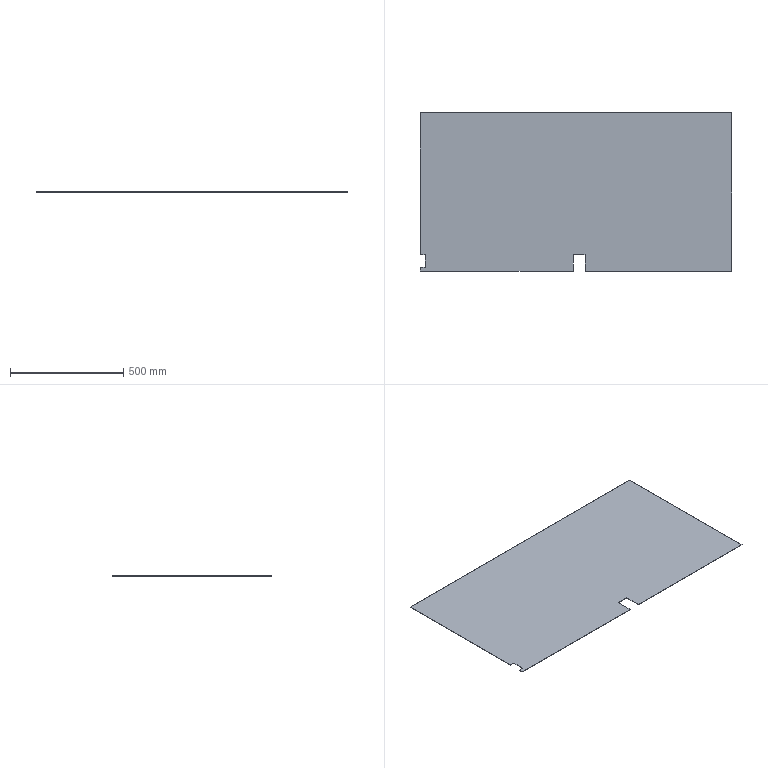Part | SolidWorks | 1 solid | 14 faces | box 1374 x 700 x 1.5 mm | volume 1435242 mm3 | plane 14
STEP:
#1=CARTESIAN_POINT('',(-687.,350.,0.));
#2=VERTEX_POINT('',#1);
#3=CARTESIAN_POINT('',(-687.,-277.,0.));
#4=VERTEX_POINT('',#3);
#5=CARTESIAN_POINT('',(-687.,-350.,0.));
#6=DIRECTION('',(0.,-1.,0.));
#7=VECTOR('',#6,1000.);
#8=LINE('',#5,#7);
#9=EDGE_CURVE('',#2,#4,#8,.T.);
#10=ORIENTED_EDGE('',*,*,#9,.T.);
#11=CARTESIAN_POINT('',(-687.,-277.,1.5));
#12=VERTEX_POINT('',#11);
#13=CARTESIAN_POINT('',(-687.,-277.,-0.001));
#14=DIRECTION('',(0.,0.,-1.));
#15=VECTOR('',#14,1000.);
#16=LINE('',#13,#15);
#17=EDGE_CURVE('',#12,#4,#16,.T.);
#18=ORIENTED_EDGE('',*,*,#17,.F.);
#19=CARTESIAN_POINT('',(-687.,350.,1.5));
#20=VERTEX_POINT('',#19);
#21=CARTESIAN_POINT('',(-687.,-350.,1.5));
#22=DIRECTION('',(0.,-1.,0.));
#23=VECTOR('',#22,1000.);
#24=LINE('',#21,#23);
#25=EDGE_CURVE('',#20,#12,#24,.T.);
#26=ORIENTED_EDGE('',*,*,#25,.F.);
#27=CARTESIAN_POINT('',(-687.,350.,1.5));
#28=DIRECTION('',(0.,0.,-1.));
#29=VECTOR('',#28,1000.);
#30=LINE('',#27,#29);
#31=EDGE_CURVE('',#20,#2,#30,.T.);
#32=ORIENTED_EDGE('',*,*,#31,.T.);
#33=EDGE_LOOP('',(#10,#18,#26,#32));
#34=FACE_OUTER_BOUND('',#33,.T.);
#35=CARTESIAN_POINT('',(-687.,-350.,1.5));
#36=DIRECTION('',(1.,0.,0.));
#37=DIRECTION('',(0.,0.,-1.));
#38=AXIS2_PLACEMENT_3D('',#35,#36,#37);
#39=PLANE('',#38);
#40=ADVANCED_FACE('',(#34),#39,.F.);
#41=CARTESIAN_POINT('',(-687.,-350.,0.));
#42=VERTEX_POINT('',#41);
#43=CARTESIAN_POINT('',(-12.,-350.,0.));
#44=VERTEX_POINT('',#43);
#45=CARTESIAN_POINT('',(687.,-350.,0.));
#46=DIRECTION('',(1.,0.,0.));
#47=VECTOR('',#46,1000.);
#48=LINE('',#45,#47);
#49=EDGE_CURVE('',#42,#44,#48,.T.);
#50=ORIENTED_EDGE('',*,*,#49,.T.);
#51=CARTESIAN_POINT('',(-12.,-350.,1.5));
#52=VERTEX_POINT('',#51);
#53=CARTESIAN_POINT('',(-12.,-350.,-0.001));
#54=DIRECTION('',(0.,0.,-1.));
#55=VECTOR('',#54,1000.);
#56=LINE('',#53,#55);
#57=EDGE_CURVE('',#52,#44,#56,.T.);
#58=ORIENTED_EDGE('',*,*,#57,.F.);
#59=CARTESIAN_POINT('',(-687.,-350.,1.5));
#60=VERTEX_POINT('',#59);
#61=CARTESIAN_POINT('',(687.,-350.,1.5));
#62=DIRECTION('',(1.,0.,0.));
#63=VECTOR('',#62,1000.);
#64=LINE('',#61,#63);
#65=EDGE_CURVE('',#60,#52,#64,.T.);
#66=ORIENTED_EDGE('',*,*,#65,.F.);
#67=CARTESIAN_POINT('',(-687.,-350.,1.5));
#68=DIRECTION('',(0.,0.,-1.));
#69=VECTOR('',#68,1000.);
#70=LINE('',#67,#69);
#71=EDGE_CURVE('',#60,#42,#70,.T.);
#72=ORIENTED_EDGE('',*,*,#71,.T.);
#73=EDGE_LOOP('',(#50,#58,#66,#72));
#74=FACE_OUTER_BOUND('',#73,.T.);
#75=CARTESIAN_POINT('',(687.,-350.,1.5));
#76=DIRECTION('',(0.,1.,0.));
#77=DIRECTION('',(0.,0.,1.));
#78=AXIS2_PLACEMENT_3D('',#75,#76,#77);
#79=PLANE('',#78);
#80=ADVANCED_FACE('',(#74),#79,.F.);
#81=CARTESIAN_POINT('',(687.,-350.,0.));
#82=VERTEX_POINT('',#81);
#83=CARTESIAN_POINT('',(687.,350.,0.));
#84=VERTEX_POINT('',#83);
#85=CARTESIAN_POINT('',(687.,-350.,0.));
#86=DIRECTION('',(0.,1.,0.));
#87=VECTOR('',#86,1000.);
#88=LINE('',#85,#87);
#89=EDGE_CURVE('',#82,#84,#88,.T.);
#90=ORIENTED_EDGE('',*,*,#89,.T.);
#91=CARTESIAN_POINT('',(687.,350.,1.5));
#92=VERTEX_POINT('',#91);
#93=CARTESIAN_POINT('',(687.,350.,1.5));
#94=DIRECTION('',(0.,0.,-1.));
#95=VECTOR('',#94,1000.);
#96=LINE('',#93,#95);
#97=EDGE_CURVE('',#92,#84,#96,.T.);
#98=ORIENTED_EDGE('',*,*,#97,.F.);
#99=CARTESIAN_POINT('',(687.,-350.,1.5));
#100=VERTEX_POINT('',#99);
#101=CARTESIAN_POINT('',(687.,-350.,1.5));
#102=DIRECTION('',(0.,1.,0.));
#103=VECTOR('',#102,1000.);
#104=LINE('',#101,#103);
#105=EDGE_CURVE('',#100,#92,#104,.T.);
#106=ORIENTED_EDGE('',*,*,#105,.F.);
#107=CARTESIAN_POINT('',(687.,-350.,1.5));
#108=DIRECTION('',(0.,0.,-1.));
#109=VECTOR('',#108,1000.);
#110=LINE('',#107,#109);
#111=EDGE_CURVE('',#100,#82,#110,.T.);
#112=ORIENTED_EDGE('',*,*,#111,.T.);
#113=EDGE_LOOP('',(#90,#98,#106,#112));
#114=FACE_OUTER_BOUND('',#113,.T.);
#115=CARTESIAN_POINT('',(687.,-350.,1.5));
#116=DIRECTION('',(-1.,0.,0.));
#117=DIRECTION('',(0.,0.,1.));
#118=AXIS2_PLACEMENT_3D('',#115,#116,#117);
#119=PLANE('',#118);
#120=ADVANCED_FACE('',(#114),#119,.F.);
#121=CARTESIAN_POINT('',(687.,350.,0.));
#122=DIRECTION('',(-1.,0.,0.));
#123=VECTOR('',#122,1000.);
#124=LINE('',#121,#123);
#125=EDGE_CURVE('',#84,#2,#124,.T.);
#126=ORIENTED_EDGE('',*,*,#125,.T.);
#127=ORIENTED_EDGE('',*,*,#31,.F.);
#128=CARTESIAN_POINT('',(687.,350.,1.5));
#129=DIRECTION('',(-1.,0.,0.));
#130=VECTOR('',#129,1000.);
#131=LINE('',#128,#130);
#132=EDGE_CURVE('',#92,#20,#131,.T.);
#133=ORIENTED_EDGE('',*,*,#132,.F.);
#134=ORIENTED_EDGE('',*,*,#97,.T.);
#135=EDGE_LOOP('',(#126,#127,#133,#134));
#136=FACE_OUTER_BOUND('',#135,.T.);
#137=CARTESIAN_POINT('',(687.,350.,1.5));
#138=DIRECTION('',(0.,-1.,0.));
#139=DIRECTION('',(0.,0.,-1.));
#140=AXIS2_PLACEMENT_3D('',#137,#138,#139);
#141=PLANE('',#140);
#142=ADVANCED_FACE('',(#136),#141,.F.);
#143=CARTESIAN_POINT('',(-687.,-333.,1.5));
#144=VERTEX_POINT('',#143);
#145=CARTESIAN_POINT('',(-687.,-350.,1.5));
#146=DIRECTION('',(0.,-1.,0.));
#147=VECTOR('',#146,1000.);
#148=LINE('',#145,#147);
#149=EDGE_CURVE('',#144,#60,#148,.T.);
#150=ORIENTED_EDGE('',*,*,#149,.F.);
#151=CARTESIAN_POINT('',(-687.,-333.,0.));
#152=VERTEX_POINT('',#151);
#153=CARTESIAN_POINT('',(-687.,-333.,-0.001));
#154=DIRECTION('',(0.,0.,1.));
#155=VECTOR('',#154,1000.);
#156=LINE('',#153,#155);
#157=EDGE_CURVE('',#152,#144,#156,.T.);
#158=ORIENTED_EDGE('',*,*,#157,.F.);
#159=CARTESIAN_POINT('',(-687.,-350.,0.));
#160=DIRECTION('',(0.,-1.,0.));
#161=VECTOR('',#160,1000.);
#162=LINE('',#159,#161);
#163=EDGE_CURVE('',#152,#42,#162,.T.);
#164=ORIENTED_EDGE('',*,*,#163,.T.);
#165=ORIENTED_EDGE('',*,*,#71,.F.);
#166=EDGE_LOOP('',(#150,#158,#164,#165));
#167=FACE_OUTER_BOUND('',#166,.T.);
#168=CARTESIAN_POINT('',(-687.,-350.,1.5));
#169=DIRECTION('',(1.,0.,0.));
#170=DIRECTION('',(0.,0.,-1.));
#171=AXIS2_PLACEMENT_3D('',#168,#169,#170);
#172=PLANE('',#171);
#173=ADVANCED_FACE('',(#167),#172,.F.);
#174=CARTESIAN_POINT('',(40.,-350.,1.5));
#175=VERTEX_POINT('',#174);
#176=CARTESIAN_POINT('',(687.,-350.,1.5));
#177=DIRECTION('',(1.,0.,0.));
#178=VECTOR('',#177,1000.);
#179=LINE('',#176,#178);
#180=EDGE_CURVE('',#175,#100,#179,.T.);
#181=ORIENTED_EDGE('',*,*,#180,.F.);
#182=CARTESIAN_POINT('',(40.,-350.,0.));
#183=VERTEX_POINT('',#182);
#184=CARTESIAN_POINT('',(40.,-350.,-0.001));
#185=DIRECTION('',(0.,0.,1.));
#186=VECTOR('',#185,1000.);
#187=LINE('',#184,#186);
#188=EDGE_CURVE('',#183,#175,#187,.T.);
#189=ORIENTED_EDGE('',*,*,#188,.F.);
#190=CARTESIAN_POINT('',(687.,-350.,0.));
#191=DIRECTION('',(1.,0.,0.));
#192=VECTOR('',#191,1000.);
#193=LINE('',#190,#192);
#194=EDGE_CURVE('',#183,#82,#193,.T.);
#195=ORIENTED_EDGE('',*,*,#194,.T.);
#196=ORIENTED_EDGE('',*,*,#111,.F.);
#197=EDGE_LOOP('',(#181,#189,#195,#196));
#198=FACE_OUTER_BOUND('',#197,.T.);
#199=CARTESIAN_POINT('',(687.,-350.,1.5));
#200=DIRECTION('',(0.,1.,0.));
#201=DIRECTION('',(0.,0.,1.));
#202=AXIS2_PLACEMENT_3D('',#199,#200,#201);
#203=PLANE('',#202);
#204=ADVANCED_FACE('',(#198),#203,.F.);
#205=CARTESIAN_POINT('',(-666.,-277.,1.5));
#206=VERTEX_POINT('',#205);
#207=CARTESIAN_POINT('',(-726.,-277.,1.5));
#208=DIRECTION('',(-1.,0.,0.));
#209=VECTOR('',#208,1000.);
#210=LINE('',#207,#209);
#211=EDGE_CURVE('',#206,#12,#210,.T.);
#212=ORIENTED_EDGE('',*,*,#211,.F.);
#213=CARTESIAN_POINT('',(-666.,-333.,1.5));
#214=VERTEX_POINT('',#213);
#215=CARTESIAN_POINT('',(-666.,-277.,1.5));
#216=DIRECTION('',(0.,1.,0.));
#217=VECTOR('',#216,1000.);
#218=LINE('',#215,#217);
#219=EDGE_CURVE('',#214,#206,#218,.T.);
#220=ORIENTED_EDGE('',*,*,#219,.F.);
#221=CARTESIAN_POINT('',(-726.,-333.,1.5));
#222=DIRECTION('',(1.,0.,0.));
#223=VECTOR('',#222,1000.);
#224=LINE('',#221,#223);
#225=EDGE_CURVE('',#144,#214,#224,.T.);
#226=ORIENTED_EDGE('',*,*,#225,.F.);
#227=ORIENTED_EDGE('',*,*,#149,.T.);
#228=ORIENTED_EDGE('',*,*,#65,.T.);
#229=CARTESIAN_POINT('',(-12.,-277.,1.5));
#230=VERTEX_POINT('',#229);
#231=CARTESIAN_POINT('',(-12.,-277.,1.5));
#232=DIRECTION('',(0.,-1.,0.));
#233=VECTOR('',#232,1000.);
#234=LINE('',#231,#233);
#235=EDGE_CURVE('',#230,#52,#234,.T.);
#236=ORIENTED_EDGE('',*,*,#235,.F.);
#237=CARTESIAN_POINT('',(40.,-277.,1.5));
#238=VERTEX_POINT('',#237);
#239=CARTESIAN_POINT('',(-12.,-277.,1.5));
#240=DIRECTION('',(-1.,0.,0.));
#241=VECTOR('',#240,1000.);
#242=LINE('',#239,#241);
#243=EDGE_CURVE('',#238,#230,#242,.T.);
#244=ORIENTED_EDGE('',*,*,#243,.F.);
#245=CARTESIAN_POINT('',(40.,-277.,1.5));
#246=DIRECTION('',(0.,1.,0.));
#247=VECTOR('',#246,1000.);
#248=LINE('',#245,#247);
#249=EDGE_CURVE('',#175,#238,#248,.T.);
#250=ORIENTED_EDGE('',*,*,#249,.F.);
#251=ORIENTED_EDGE('',*,*,#180,.T.);
#252=ORIENTED_EDGE('',*,*,#105,.T.);
#253=ORIENTED_EDGE('',*,*,#132,.T.);
#254=ORIENTED_EDGE('',*,*,#25,.T.);
#255=EDGE_LOOP('',(#212,#220,#226,#227,#228,#236,#244,#250,#251,#252,#253,#254));
#256=FACE_OUTER_BOUND('',#255,.T.);
#257=CARTESIAN_POINT('',(0.,0.,1.5));
#258=DIRECTION('',(0.,0.,1.));
#259=DIRECTION('',(1.,0.,0.));
#260=AXIS2_PLACEMENT_3D('',#257,#258,#259);
#261=PLANE('',#260);
#262=ADVANCED_FACE('',(#256),#261,.T.);
#263=CARTESIAN_POINT('',(-666.,-277.,0.));
#264=VERTEX_POINT('',#263);
#265=CARTESIAN_POINT('',(-666.,-333.,0.));
#266=VERTEX_POINT('',#265);
#267=CARTESIAN_POINT('',(-666.,-277.,0.));
#268=DIRECTION('',(0.,-1.,0.));
#269=VECTOR('',#268,1000.);
#270=LINE('',#267,#269);
#271=EDGE_CURVE('',#264,#266,#270,.T.);
#272=ORIENTED_EDGE('',*,*,#271,.F.);
#273=CARTESIAN_POINT('',(-726.,-277.,0.));
#274=DIRECTION('',(1.,0.,0.));
#275=VECTOR('',#274,1000.);
#276=LINE('',#273,#275);
#277=EDGE_CURVE('',#4,#264,#276,.T.);
#278=ORIENTED_EDGE('',*,*,#277,.F.);
#279=ORIENTED_EDGE('',*,*,#9,.F.);
#280=ORIENTED_EDGE('',*,*,#125,.F.);
#281=ORIENTED_EDGE('',*,*,#89,.F.);
#282=ORIENTED_EDGE('',*,*,#194,.F.);
#283=CARTESIAN_POINT('',(40.,-277.,0.));
#284=VERTEX_POINT('',#283);
#285=CARTESIAN_POINT('',(40.,-277.,0.));
#286=DIRECTION('',(0.,-1.,0.));
#287=VECTOR('',#286,1000.);
#288=LINE('',#285,#287);
#289=EDGE_CURVE('',#284,#183,#288,.T.);
#290=ORIENTED_EDGE('',*,*,#289,.F.);
#291=CARTESIAN_POINT('',(-12.,-277.,0.));
#292=VERTEX_POINT('',#291);
#293=CARTESIAN_POINT('',(-12.,-277.,0.));
#294=DIRECTION('',(1.,0.,0.));
#295=VECTOR('',#294,1000.);
#296=LINE('',#293,#295);
#297=EDGE_CURVE('',#292,#284,#296,.T.);
#298=ORIENTED_EDGE('',*,*,#297,.F.);
#299=CARTESIAN_POINT('',(-12.,-277.,0.));
#300=DIRECTION('',(0.,1.,0.));
#301=VECTOR('',#300,1000.);
#302=LINE('',#299,#301);
#303=EDGE_CURVE('',#44,#292,#302,.T.);
#304=ORIENTED_EDGE('',*,*,#303,.F.);
#305=ORIENTED_EDGE('',*,*,#49,.F.);
#306=ORIENTED_EDGE('',*,*,#163,.F.);
#307=CARTESIAN_POINT('',(-726.,-333.,0.));
#308=DIRECTION('',(-1.,0.,0.));
#309=VECTOR('',#308,1000.);
#310=LINE('',#307,#309);
#311=EDGE_CURVE('',#266,#152,#310,.T.);
#312=ORIENTED_EDGE('',*,*,#311,.F.);
#313=EDGE_LOOP('',(#272,#278,#279,#280,#281,#282,#290,#298,#304,#305,#306,#312));
#314=FACE_OUTER_BOUND('',#313,.T.);
#315=CARTESIAN_POINT('',(0.,0.,0.));
#316=DIRECTION('',(0.,0.,1.));
#317=DIRECTION('',(1.,0.,0.));
#318=AXIS2_PLACEMENT_3D('',#315,#316,#317);
#319=PLANE('',#318);
#320=ADVANCED_FACE('',(#314),#319,.F.);
#321=ORIENTED_EDGE('',*,*,#57,.T.);
#322=ORIENTED_EDGE('',*,*,#303,.T.);
#323=CARTESIAN_POINT('',(-12.,-277.,-0.001));
#324=DIRECTION('',(0.,0.,1.));
#325=VECTOR('',#324,1000.);
#326=LINE('',#323,#325);
#327=EDGE_CURVE('',#292,#230,#326,.T.);
#328=ORIENTED_EDGE('',*,*,#327,.T.);
#329=ORIENTED_EDGE('',*,*,#235,.T.);
#330=EDGE_LOOP('',(#321,#322,#328,#329));
#331=FACE_OUTER_BOUND('',#330,.T.);
#332=CARTESIAN_POINT('',(-12.,-277.,-0.001));
#333=DIRECTION('',(-1.,0.,0.));
#334=DIRECTION('',(0.,-1.,0.));
#335=AXIS2_PLACEMENT_3D('',#332,#333,#334);
#336=PLANE('',#335);
#337=ADVANCED_FACE('',(#331),#336,.F.);
#338=ORIENTED_EDGE('',*,*,#297,.T.);
#339=CARTESIAN_POINT('',(40.,-277.,-0.001));
#340=DIRECTION('',(0.,0.,1.));
#341=VECTOR('',#340,1000.);
#342=LINE('',#339,#341);
#343=EDGE_CURVE('',#284,#238,#342,.T.);
#344=ORIENTED_EDGE('',*,*,#343,.T.);
#345=ORIENTED_EDGE('',*,*,#243,.T.);
#346=ORIENTED_EDGE('',*,*,#327,.F.);
#347=EDGE_LOOP('',(#338,#344,#345,#346));
#348=FACE_OUTER_BOUND('',#347,.T.);
#349=CARTESIAN_POINT('',(-12.,-277.,-0.001));
#350=DIRECTION('',(0.,1.,0.));
#351=DIRECTION('',(0.,0.,1.));
#352=AXIS2_PLACEMENT_3D('',#349,#350,#351);
#353=PLANE('',#352);
#354=ADVANCED_FACE('',(#348),#353,.F.);
#355=ORIENTED_EDGE('',*,*,#188,.T.);
#356=ORIENTED_EDGE('',*,*,#249,.T.);
#357=ORIENTED_EDGE('',*,*,#343,.F.);
#358=ORIENTED_EDGE('',*,*,#289,.T.);
#359=EDGE_LOOP('',(#355,#356,#357,#358));
#360=FACE_OUTER_BOUND('',#359,.T.);
#361=CARTESIAN_POINT('',(40.,-277.,-0.001));
#362=DIRECTION('',(1.,0.,0.));
#363=DIRECTION('',(0.,1.,0.));
#364=AXIS2_PLACEMENT_3D('',#361,#362,#363);
#365=PLANE('',#364);
#366=ADVANCED_FACE('',(#360),#365,.F.);
#367=ORIENTED_EDGE('',*,*,#17,.T.);
#368=ORIENTED_EDGE('',*,*,#277,.T.);
#369=CARTESIAN_POINT('',(-666.,-277.,-0.001));
#370=DIRECTION('',(0.,0.,1.));
#371=VECTOR('',#370,1000.);
#372=LINE('',#369,#371);
#373=EDGE_CURVE('',#264,#206,#372,.T.);
#374=ORIENTED_EDGE('',*,*,#373,.T.);
#375=ORIENTED_EDGE('',*,*,#211,.T.);
#376=EDGE_LOOP('',(#367,#368,#374,#375));
#377=FACE_OUTER_BOUND('',#376,.T.);
#378=CARTESIAN_POINT('',(-726.,-277.,-0.001));
#379=DIRECTION('',(0.,1.,0.));
#380=DIRECTION('',(0.,0.,1.));
#381=AXIS2_PLACEMENT_3D('',#378,#379,#380);
#382=PLANE('',#381);
#383=ADVANCED_FACE('',(#377),#382,.F.);
#384=ORIENTED_EDGE('',*,*,#271,.T.);
#385=CARTESIAN_POINT('',(-666.,-333.,-0.001));
#386=DIRECTION('',(0.,0.,1.));
#387=VECTOR('',#386,1000.);
#388=LINE('',#385,#387);
#389=EDGE_CURVE('',#266,#214,#388,.T.);
#390=ORIENTED_EDGE('',*,*,#389,.T.);
#391=ORIENTED_EDGE('',*,*,#219,.T.);
#392=ORIENTED_EDGE('',*,*,#373,.F.);
#393=EDGE_LOOP('',(#384,#390,#391,#392));
#394=FACE_OUTER_BOUND('',#393,.T.);
#395=CARTESIAN_POINT('',(-666.,-277.,-0.001));
#396=DIRECTION('',(1.,0.,0.));
#397=DIRECTION('',(0.,0.,-1.));
#398=AXIS2_PLACEMENT_3D('',#395,#396,#397);
#399=PLANE('',#398);
#400=ADVANCED_FACE('',(#394),#399,.F.);
#401=ORIENTED_EDGE('',*,*,#157,.T.);
#402=ORIENTED_EDGE('',*,*,#225,.T.);
#403=ORIENTED_EDGE('',*,*,#389,.F.);
#404=ORIENTED_EDGE('',*,*,#311,.T.);
#405=EDGE_LOOP('',(#401,#402,#403,#404));
#406=FACE_OUTER_BOUND('',#405,.T.);
#407=CARTESIAN_POINT('',(-726.,-333.,-0.001));
#408=DIRECTION('',(0.,-1.,0.));
#409=DIRECTION('',(0.,0.,-1.));
#410=AXIS2_PLACEMENT_3D('',#407,#408,#409);
#411=PLANE('',#410);
#412=ADVANCED_FACE('',(#406),#411,.F.);
#413=CLOSED_SHELL('',(#40,#80,#120,#142,#173,#204,#262,#320,#337,#354,#366,#383,#400,#412));
#414=MANIFOLD_SOLID_BREP('',#413);
#415=CARTESIAN_POINT('',(0.,0.,0.));
#416=DIRECTION('',(0.,0.,1.));
#417=DIRECTION('',(1.,0.,0.));
#418=AXIS2_PLACEMENT_3D('',#415,#416,#417);
#419=(LENGTH_UNIT()NAMED_UNIT(*)SI_UNIT(.MILLI.,.METRE.));
#420=UNCERTAINTY_MEASURE_WITH_UNIT(LENGTH_MEASURE(0.00001),#419,'','');
#421=(NAMED_UNIT(*)PLANE_ANGLE_UNIT()SI_UNIT($,.RADIAN.));
#422=(NAMED_UNIT(*)SI_UNIT($,.STERADIAN.)SOLID_ANGLE_UNIT());
#423=(GEOMETRIC_REPRESENTATION_CONTEXT(3)GLOBAL_UNCERTAINTY_ASSIGNED_CONTEXT((#420))GLOBAL_UNIT_ASSIGNED_CONTEXT((#419,#421,#422))REPRESENTATION_CONTEXT('',''));
#424=ADVANCED_BREP_SHAPE_REPRESENTATION('',(#414,#418),#423);